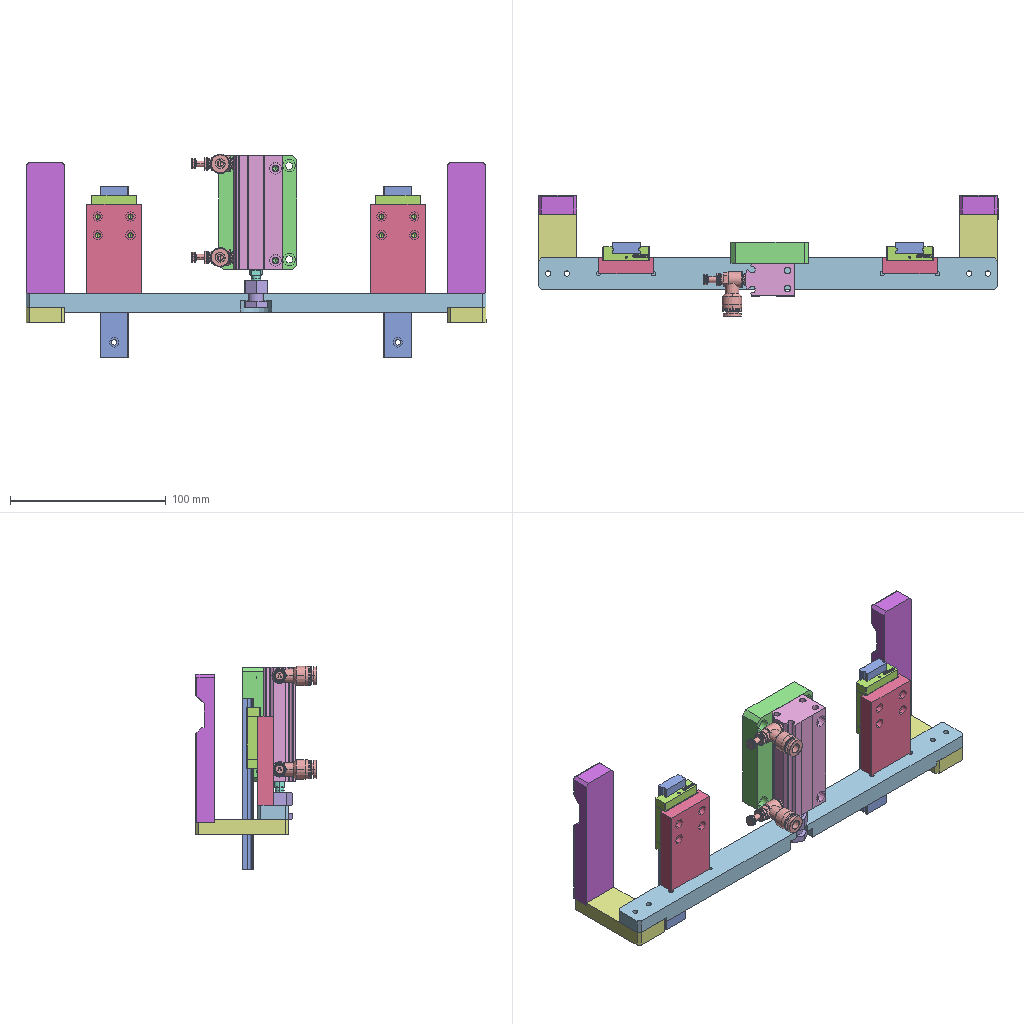Assembly | SolidWorks | 10 different items | 16 placed | box 295 x 78 x 131 mm
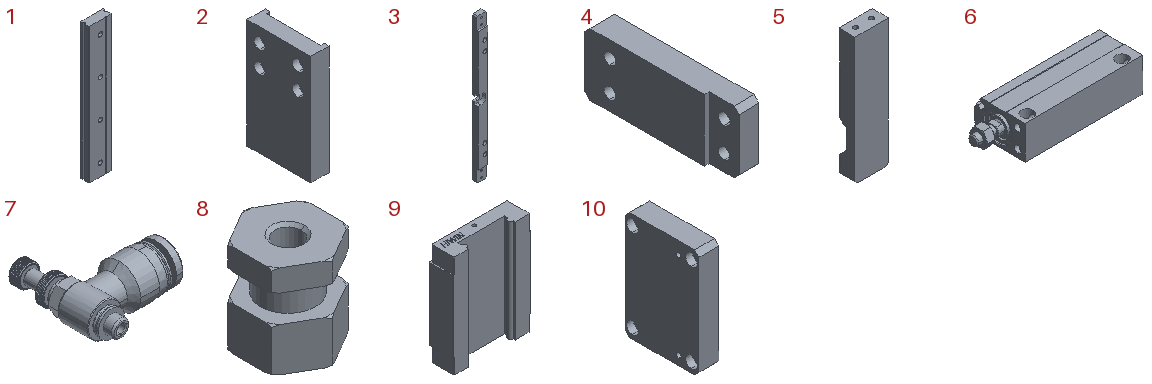Parts list (item | quantity | size | volume | features):
1 | x2 | 18 x 7 x 110 mm | 12871 mm3 | features Extrusion 1, HoleWzd 1, ICE 1, LPattern 1
2 | x2 | 10 x 35 x 60 mm | 16670 mm3 | features HoleWzd 2, Cut 1, Extrusion 1
3 | x1 | 20 x 12 x 295 mm | 61579 mm3 | features HoleWzd 3, ICE 3, Cut 2, Chamfer 1, Extrusion 1
4 | x2 | 10 x 60 x 25 mm | 13123 mm3 | features HoleWzd 2, Chamfer 1, Extrusion 1, ICE 1
5 | x2 | 25 x 12 x 95 mm | 25505 mm3 | features Chamfer 2, Cut 1, Extrusion 1, Fillet 1, HoleWzd 1, ICE 1
6 | x1 | 89 x 31.5 x 21 mm | 33779 mm3 | features BaseBody 3
7 | x2 | 28.6 x 30 x 12.5 mm | 2558 mm3 | features BaseBody 1
8 | x1 | 14 x 16.166 x 17 mm | 2101 mm3 | features BaseBody 1
9 | x2 | 30 x 9.1 x 39.3 mm | 7510 mm3 | features BaseBody 1
10 | x1 | 13.5 x 50 x 73.5 mm | 47539 mm3 | features HoleWzd 3, Chamfer 1, Extrusion 1
Mates (type | each side: item.copy, entity, surface, feature):
Concentric | 6.1 face cylinder _MU16X50S_body-1-solid1 | 7.1 face cylinder Import1
Coincident | 6.1 face plane _MU16X50S_body-1-solid1 | 7.1 face plane Import1
Parallel | 6.1 face plane _MU16X50S_body-1-solid1 | 7.1 face plane Import1
Concentric | 6.1 face cylinder _MU16X50S_body-1-solid1 | 7.2 face cylinder Import1
Coincident | 6.1 face plane _MU16X50S_body-1-solid1 | 7.2 face plane Import1
Parallel | 6.1 face plane _MU16X50S_body-1-solid1 | 7.2 face plane Import1
Coincident | 9.1 face plane Import2 | 1.1 face plane Boss-Extrude1
Width | 9.1 face plane Import2 | 9.1 face plane Import2 | 1.1 face plane Boss-Extrude1 | 1.1 face plane Boss-Extrude1
Coincident | 1.1 face plane Boss-Extrude1 | 1.2 face plane Boss-Extrude1
Coincident | 1.2 face plane Boss-Extrude1 | 9.2 face plane Import2
Width | 9.2 face plane Import2 | 9.2 face plane Import2 | 1.2 face plane Boss-Extrude1 | 1.2 face plane Boss-Extrude1
Width | 9.1 face plane Import2 | 9.1 face plane Import2 | 2.1 face plane Boss-Extrude1 | 2.1 face plane Boss-Extrude1
Coincident | 2.1 face plane Boss-Extrude1 | 9.1 face plane Import2
Coincident | 2.1 face plane Cut-Extrude1 | 9.1 face plane Import2
Width | 9.2 face plane Import2 | 9.2 face plane Import2 | 2.2 face plane Boss-Extrude1 | 2.2 face plane Boss-Extrude1
Coincident | 2.2 face plane Boss-Extrude1 | 9.2 face plane Import2
Coincident | 2.2 face plane Cut-Extrude1 | 9.2 face plane Import2
Width | 3.1 face plane Boss-Extrude1 | 3.1 face plane Boss-Extrude1 | 6.1 face cylinder _MU16X50SB_rod-1-solid1
Concentric | 6.1 face cylinder _MU16X50SB_rod-1-solid1 | 8.1 face cylinder Import1
Coincident | 6.1 face plane _16_nut-1-solid1 | 8.1 face plane Import1
Coincident | 6.1 face plane _MU16X50S_body-1-solid1 | 10.1 face plane Boss-Extrude1
Width | 10.1 face plane Boss-Extrude1 | 10.1 face plane Boss-Extrude1 | 6.1 face plane _MU16X50S_body-1-solid1 | 6.1 face plane _MU16X50S_body-1-solid1
Concentric | 3.1 face cylinder Cut-Extrude1 | 8.1 face cylinder Import1
LimitDistanceDim | 3.1 face plane Boss-Extrude1 | 8.1 face plane Import1
Coincident | 3.1 face plane Cut-Extrude4 | 2.1 face plane Boss-Extrude1
Coincident | 3.1 face plane Cut-Extrude4 | 2.2 face plane Boss-Extrude1
Coincident | 3.1 face plane Cut-Extrude3 | 4.1 face plane Boss-Extrude1
Coincident | 3.1 face plane Boss-Extrude1 | 4.1 face plane Boss-Extrude1 | 2 times
Coincident | 5.1 face plane Boss-Extrude1 | 4.2 face plane Cut-Extrude3
Coincident | 5.1 face plane Boss-Extrude1 | 4.2 face plane Boss-Extrude1 | 2 times
Coincident | 5.2 face plane Boss-Extrude1 | 4.1 face plane Cut-Extrude3
Coincident | 5.2 face plane Boss-Extrude1 | 4.1 face plane Boss-Extrude1 | 2 times
Coincident | 5.1 face plane Boss-Extrude1 | 5.2 face plane Boss-Extrude1 | 2 times